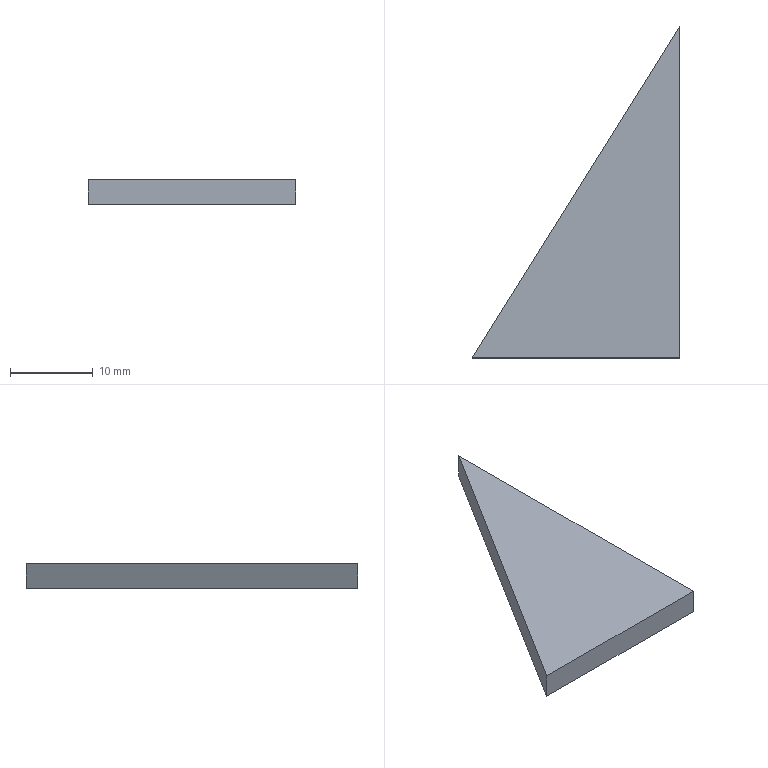Part | STEP file | Q7C0109 | 1 solid | 5 faces | box 25 x 40 x 3 mm | volume 1500 mm3 | plane 5
STEP:
#1=CARTESIAN_POINT('',(0.,0.,0.));
#2=DIRECTION('',(0.,0.,1.));
#3=DIRECTION('',(1.,0.,0.));
#4=AXIS2_PLACEMENT_3D('',#1,#2,#3);
#5=CARTESIAN_POINT('',(-25.,0.,0.));
#6=VERTEX_POINT('',#5);
#7=CARTESIAN_POINT('',(0.,0.,0.));
#8=VERTEX_POINT('',#7);
#9=CARTESIAN_POINT('',(-25.,0.,0.));
#10=DIRECTION('',(1.,0.,0.));
#11=VECTOR('',#10,1.);
#12=LINE('',#9,#11);
#13=CARTESIAN_POINT('',(-25.,0.,3.));
#14=DIRECTION('',(0.,1.,0.));
#15=DIRECTION('',(0.,0.,1.));
#16=AXIS2_PLACEMENT_3D('',#13,#14,#15);
#17=PLANE('',#16);
#18=CARTESIAN_POINT('',(-3.,0.));
#19=DIRECTION('',(0.,1.));
#20=VECTOR('',#19,1.);
#21=LINE('',#18,#20);
#22=(GEOMETRIC_REPRESENTATION_CONTEXT(2)PARAMETRIC_REPRESENTATION_CONTEXT()REPRESENTATION_CONTEXT('',''));
#23=DEFINITIONAL_REPRESENTATION('',(#21),#22);
#24=PCURVE('',#17,#23);
#25=CARTESIAN_POINT('',(0.,0.,0.));
#26=DIRECTION('',(0.,0.,1.));
#27=DIRECTION('',(1.,0.,0.));
#28=AXIS2_PLACEMENT_3D('',#25,#26,#27);
#29=PLANE('',#28);
#30=CARTESIAN_POINT('',(-25.,0.));
#31=DIRECTION('',(1.,0.));
#32=VECTOR('',#31,1.);
#33=LINE('',#30,#32);
#34=(GEOMETRIC_REPRESENTATION_CONTEXT(2)PARAMETRIC_REPRESENTATION_CONTEXT()REPRESENTATION_CONTEXT('',''));
#35=DEFINITIONAL_REPRESENTATION('',(#33),#34);
#36=PCURVE('',#29,#35);
#37=SURFACE_CURVE('',#12,(#24,#36),.PCURVE_S1.);
#38=EDGE_CURVE('',#6,#8,#37,.T.);
#39=ORIENTED_EDGE('',*,*,#38,.T.);
#40=CARTESIAN_POINT('',(0.,0.,3.));
#41=VERTEX_POINT('',#40);
#42=CARTESIAN_POINT('',(0.,0.,3.));
#43=DIRECTION('',(0.,0.,-1.));
#44=VECTOR('',#43,1.);
#45=LINE('',#42,#44);
#46=CARTESIAN_POINT('',(0.,25.));
#47=DIRECTION('',(-1.,0.));
#48=VECTOR('',#47,1.);
#49=LINE('',#46,#48);
#50=(GEOMETRIC_REPRESENTATION_CONTEXT(2)PARAMETRIC_REPRESENTATION_CONTEXT()REPRESENTATION_CONTEXT('',''));
#51=DEFINITIONAL_REPRESENTATION('',(#49),#50);
#52=PCURVE('',#17,#51);
#53=CARTESIAN_POINT('',(0.,0.,3.));
#54=DIRECTION('',(-1.,0.,0.));
#55=DIRECTION('',(0.,0.,1.));
#56=AXIS2_PLACEMENT_3D('',#53,#54,#55);
#57=PLANE('',#56);
#58=CARTESIAN_POINT('',(0.,0.));
#59=DIRECTION('',(-1.,0.));
#60=VECTOR('',#59,1.);
#61=LINE('',#58,#60);
#62=(GEOMETRIC_REPRESENTATION_CONTEXT(2)PARAMETRIC_REPRESENTATION_CONTEXT()REPRESENTATION_CONTEXT('',''));
#63=DEFINITIONAL_REPRESENTATION('',(#61),#62);
#64=PCURVE('',#57,#63);
#65=SURFACE_CURVE('',#45,(#52,#64),.PCURVE_S1.);
#66=EDGE_CURVE('',#41,#8,#65,.T.);
#67=ORIENTED_EDGE('',*,*,#66,.F.);
#68=CARTESIAN_POINT('',(-25.,0.,3.));
#69=VERTEX_POINT('',#68);
#70=CARTESIAN_POINT('',(-25.,0.,3.));
#71=DIRECTION('',(1.,0.,0.));
#72=VECTOR('',#71,1.);
#73=LINE('',#70,#72);
#74=CARTESIAN_POINT('',(0.,0.));
#75=DIRECTION('',(0.,1.));
#76=VECTOR('',#75,1.);
#77=LINE('',#74,#76);
#78=(GEOMETRIC_REPRESENTATION_CONTEXT(2)PARAMETRIC_REPRESENTATION_CONTEXT()REPRESENTATION_CONTEXT('',''));
#79=DEFINITIONAL_REPRESENTATION('',(#77),#78);
#80=PCURVE('',#17,#79);
#81=CARTESIAN_POINT('',(0.,0.,3.));
#82=DIRECTION('',(0.,0.,1.));
#83=DIRECTION('',(1.,0.,0.));
#84=AXIS2_PLACEMENT_3D('',#81,#82,#83);
#85=PLANE('',#84);
#86=CARTESIAN_POINT('',(-25.,0.));
#87=DIRECTION('',(1.,0.));
#88=VECTOR('',#87,1.);
#89=LINE('',#86,#88);
#90=(GEOMETRIC_REPRESENTATION_CONTEXT(2)PARAMETRIC_REPRESENTATION_CONTEXT()REPRESENTATION_CONTEXT('',''));
#91=DEFINITIONAL_REPRESENTATION('',(#89),#90);
#92=PCURVE('',#85,#91);
#93=SURFACE_CURVE('',#73,(#80,#92),.PCURVE_S1.);
#94=EDGE_CURVE('',#69,#41,#93,.T.);
#95=ORIENTED_EDGE('',*,*,#94,.F.);
#96=CARTESIAN_POINT('',(-25.,0.,3.));
#97=DIRECTION('',(0.,0.,-1.));
#98=VECTOR('',#97,1.);
#99=LINE('',#96,#98);
#100=CARTESIAN_POINT('',(0.,0.));
#101=DIRECTION('',(-1.,0.));
#102=VECTOR('',#101,1.);
#103=LINE('',#100,#102);
#104=(GEOMETRIC_REPRESENTATION_CONTEXT(2)PARAMETRIC_REPRESENTATION_CONTEXT()REPRESENTATION_CONTEXT('',''));
#105=DEFINITIONAL_REPRESENTATION('',(#103),#104);
#106=PCURVE('',#17,#105);
#107=CARTESIAN_POINT('',(0.,40.,3.));
#108=DIRECTION('',(0.848,-0.53,0.));
#109=DIRECTION('',(0.53,0.848,0.));
#110=AXIS2_PLACEMENT_3D('',#107,#108,#109);
#111=PLANE('',#110);
#112=CARTESIAN_POINT('',(-47.17,0.));
#113=DIRECTION('',(0.,-1.));
#114=VECTOR('',#113,1.);
#115=LINE('',#112,#114);
#116=(GEOMETRIC_REPRESENTATION_CONTEXT(2)PARAMETRIC_REPRESENTATION_CONTEXT()REPRESENTATION_CONTEXT('',''));
#117=DEFINITIONAL_REPRESENTATION('',(#115),#116);
#118=PCURVE('',#111,#117);
#119=SURFACE_CURVE('',#99,(#106,#118),.PCURVE_S1.);
#120=EDGE_CURVE('',#69,#6,#119,.T.);
#121=ORIENTED_EDGE('',*,*,#120,.T.);
#122=EDGE_LOOP('',(#39,#67,#95,#121));
#123=FACE_BOUND('',#122,.T.);
#124=ADVANCED_FACE('',(#123),#17,.F.);
#125=CARTESIAN_POINT('',(0.,40.,0.));
#126=VERTEX_POINT('',#125);
#127=CARTESIAN_POINT('',(0.,0.,0.));
#128=DIRECTION('',(0.,1.,0.));
#129=VECTOR('',#128,1.);
#130=LINE('',#127,#129);
#131=CARTESIAN_POINT('',(-3.,0.));
#132=DIRECTION('',(0.,1.));
#133=VECTOR('',#132,1.);
#134=LINE('',#131,#133);
#135=(GEOMETRIC_REPRESENTATION_CONTEXT(2)PARAMETRIC_REPRESENTATION_CONTEXT()REPRESENTATION_CONTEXT('',''));
#136=DEFINITIONAL_REPRESENTATION('',(#134),#135);
#137=PCURVE('',#57,#136);
#138=CARTESIAN_POINT('',(0.,0.));
#139=DIRECTION('',(0.,1.));
#140=VECTOR('',#139,1.);
#141=LINE('',#138,#140);
#142=(GEOMETRIC_REPRESENTATION_CONTEXT(2)PARAMETRIC_REPRESENTATION_CONTEXT()REPRESENTATION_CONTEXT('',''));
#143=DEFINITIONAL_REPRESENTATION('',(#141),#142);
#144=PCURVE('',#29,#143);
#145=SURFACE_CURVE('',#130,(#137,#144),.PCURVE_S1.);
#146=EDGE_CURVE('',#8,#126,#145,.T.);
#147=ORIENTED_EDGE('',*,*,#146,.T.);
#148=CARTESIAN_POINT('',(0.,40.,3.));
#149=VERTEX_POINT('',#148);
#150=CARTESIAN_POINT('',(0.,40.,3.));
#151=DIRECTION('',(0.,0.,-1.));
#152=VECTOR('',#151,1.);
#153=LINE('',#150,#152);
#154=CARTESIAN_POINT('',(0.,40.));
#155=DIRECTION('',(-1.,0.));
#156=VECTOR('',#155,1.);
#157=LINE('',#154,#156);
#158=(GEOMETRIC_REPRESENTATION_CONTEXT(2)PARAMETRIC_REPRESENTATION_CONTEXT()REPRESENTATION_CONTEXT('',''));
#159=DEFINITIONAL_REPRESENTATION('',(#157),#158);
#160=PCURVE('',#57,#159);
#161=CARTESIAN_POINT('',(0.,0.));
#162=DIRECTION('',(0.,-1.));
#163=VECTOR('',#162,1.);
#164=LINE('',#161,#163);
#165=(GEOMETRIC_REPRESENTATION_CONTEXT(2)PARAMETRIC_REPRESENTATION_CONTEXT()REPRESENTATION_CONTEXT('',''));
#166=DEFINITIONAL_REPRESENTATION('',(#164),#165);
#167=PCURVE('',#111,#166);
#168=SURFACE_CURVE('',#153,(#160,#167),.PCURVE_S1.);
#169=EDGE_CURVE('',#149,#126,#168,.T.);
#170=ORIENTED_EDGE('',*,*,#169,.F.);
#171=CARTESIAN_POINT('',(0.,0.,3.));
#172=DIRECTION('',(0.,1.,0.));
#173=VECTOR('',#172,1.);
#174=LINE('',#171,#173);
#175=CARTESIAN_POINT('',(0.,0.));
#176=DIRECTION('',(0.,1.));
#177=VECTOR('',#176,1.);
#178=LINE('',#175,#177);
#179=(GEOMETRIC_REPRESENTATION_CONTEXT(2)PARAMETRIC_REPRESENTATION_CONTEXT()REPRESENTATION_CONTEXT('',''));
#180=DEFINITIONAL_REPRESENTATION('',(#178),#179);
#181=PCURVE('',#57,#180);
#182=CARTESIAN_POINT('',(0.,0.));
#183=DIRECTION('',(0.,1.));
#184=VECTOR('',#183,1.);
#185=LINE('',#182,#184);
#186=(GEOMETRIC_REPRESENTATION_CONTEXT(2)PARAMETRIC_REPRESENTATION_CONTEXT()REPRESENTATION_CONTEXT('',''));
#187=DEFINITIONAL_REPRESENTATION('',(#185),#186);
#188=PCURVE('',#85,#187);
#189=SURFACE_CURVE('',#174,(#181,#188),.PCURVE_S1.);
#190=EDGE_CURVE('',#41,#149,#189,.T.);
#191=ORIENTED_EDGE('',*,*,#190,.F.);
#192=ORIENTED_EDGE('',*,*,#66,.T.);
#193=EDGE_LOOP('',(#147,#170,#191,#192));
#194=FACE_BOUND('',#193,.T.);
#195=ADVANCED_FACE('',(#194),#57,.F.);
#196=CARTESIAN_POINT('',(0.,40.,0.));
#197=DIRECTION('',(-0.53,-0.848,0.));
#198=VECTOR('',#197,1.);
#199=LINE('',#196,#198);
#200=CARTESIAN_POINT('',(0.,-3.));
#201=DIRECTION('',(-1.,0.));
#202=VECTOR('',#201,1.);
#203=LINE('',#200,#202);
#204=(GEOMETRIC_REPRESENTATION_CONTEXT(2)PARAMETRIC_REPRESENTATION_CONTEXT()REPRESENTATION_CONTEXT('',''));
#205=DEFINITIONAL_REPRESENTATION('',(#203),#204);
#206=PCURVE('',#111,#205);
#207=CARTESIAN_POINT('',(0.,40.));
#208=DIRECTION('',(-0.53,-0.848));
#209=VECTOR('',#208,1.);
#210=LINE('',#207,#209);
#211=(GEOMETRIC_REPRESENTATION_CONTEXT(2)PARAMETRIC_REPRESENTATION_CONTEXT()REPRESENTATION_CONTEXT('',''));
#212=DEFINITIONAL_REPRESENTATION('',(#210),#211);
#213=PCURVE('',#29,#212);
#214=SURFACE_CURVE('',#199,(#206,#213),.PCURVE_S1.);
#215=EDGE_CURVE('',#126,#6,#214,.T.);
#216=ORIENTED_EDGE('',*,*,#215,.T.);
#217=ORIENTED_EDGE('',*,*,#120,.F.);
#218=CARTESIAN_POINT('',(0.,40.,3.));
#219=DIRECTION('',(-0.53,-0.848,0.));
#220=VECTOR('',#219,1.);
#221=LINE('',#218,#220);
#222=CARTESIAN_POINT('',(0.,0.));
#223=DIRECTION('',(-1.,0.));
#224=VECTOR('',#223,1.);
#225=LINE('',#222,#224);
#226=(GEOMETRIC_REPRESENTATION_CONTEXT(2)PARAMETRIC_REPRESENTATION_CONTEXT()REPRESENTATION_CONTEXT('',''));
#227=DEFINITIONAL_REPRESENTATION('',(#225),#226);
#228=PCURVE('',#111,#227);
#229=CARTESIAN_POINT('',(0.,40.));
#230=DIRECTION('',(-0.53,-0.848));
#231=VECTOR('',#230,1.);
#232=LINE('',#229,#231);
#233=(GEOMETRIC_REPRESENTATION_CONTEXT(2)PARAMETRIC_REPRESENTATION_CONTEXT()REPRESENTATION_CONTEXT('',''));
#234=DEFINITIONAL_REPRESENTATION('',(#232),#233);
#235=PCURVE('',#85,#234);
#236=SURFACE_CURVE('',#221,(#228,#235),.PCURVE_S1.);
#237=EDGE_CURVE('',#149,#69,#236,.T.);
#238=ORIENTED_EDGE('',*,*,#237,.F.);
#239=ORIENTED_EDGE('',*,*,#169,.T.);
#240=EDGE_LOOP('',(#216,#217,#238,#239));
#241=FACE_BOUND('',#240,.T.);
#242=ADVANCED_FACE('',(#241),#111,.F.);
#243=ORIENTED_EDGE('',*,*,#94,.T.);
#244=ORIENTED_EDGE('',*,*,#190,.T.);
#245=ORIENTED_EDGE('',*,*,#237,.T.);
#246=EDGE_LOOP('',(#243,#244,#245));
#247=FACE_BOUND('',#246,.T.);
#248=ADVANCED_FACE('',(#247),#85,.T.);
#249=ORIENTED_EDGE('',*,*,#38,.F.);
#250=ORIENTED_EDGE('',*,*,#215,.F.);
#251=ORIENTED_EDGE('',*,*,#146,.F.);
#252=EDGE_LOOP('',(#249,#250,#251));
#253=FACE_BOUND('',#252,.T.);
#254=ADVANCED_FACE('',(#253),#29,.F.);
#255=CLOSED_SHELL('',(#124,#195,#242,#248,#254));
#256=MANIFOLD_SOLID_BREP('',#255);
#257=(LENGTH_UNIT()NAMED_UNIT(*)SI_UNIT(.MILLI.,.METRE.));
#258=UNCERTAINTY_MEASURE_WITH_UNIT(LENGTH_MEASURE(0.0000001),#257,'','');
#259=(NAMED_UNIT(*)PLANE_ANGLE_UNIT()SI_UNIT($,.RADIAN.));
#260=(NAMED_UNIT(*)SI_UNIT($,.STERADIAN.)SOLID_ANGLE_UNIT());
#261=(GEOMETRIC_REPRESENTATION_CONTEXT(3)GLOBAL_UNCERTAINTY_ASSIGNED_CONTEXT((#258))GLOBAL_UNIT_ASSIGNED_CONTEXT((#257,#259,#260))REPRESENTATION_CONTEXT('',''));
#262=ADVANCED_BREP_SHAPE_REPRESENTATION('',(#4,#256),#261);